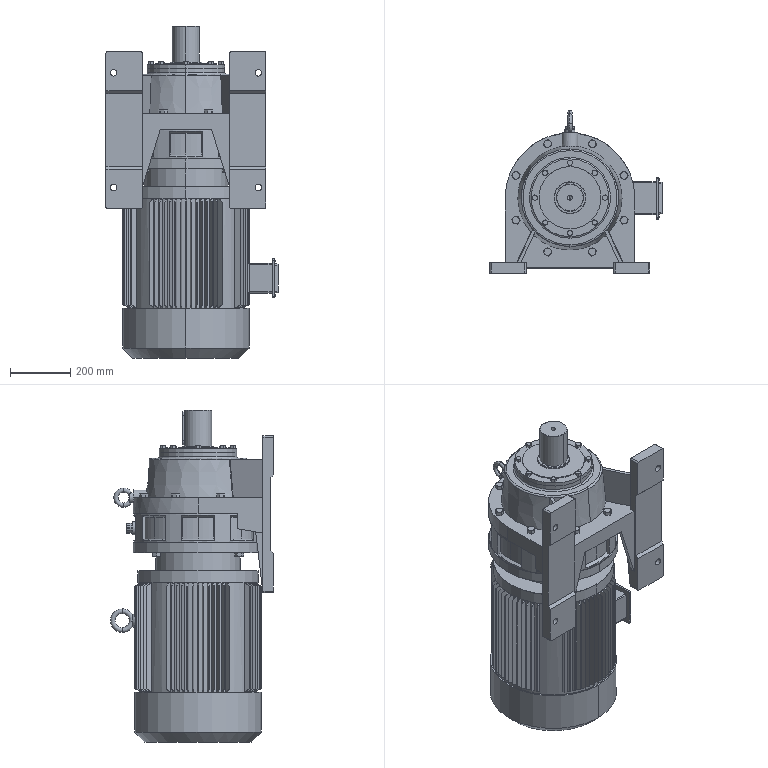Part | SolidWorks | 4 solids | 997 faces | box 570 x 540.12 x 1100 mm | volume 120754101 mm3 | plane 575 | cylinder 215 | cone 185 | torus 14 | spline 6 | sphere 2 | commonest cylinder face diameters 420 x63 4.455 x20 1 x19 405.269 x16 8.91 x12 32.797 x12